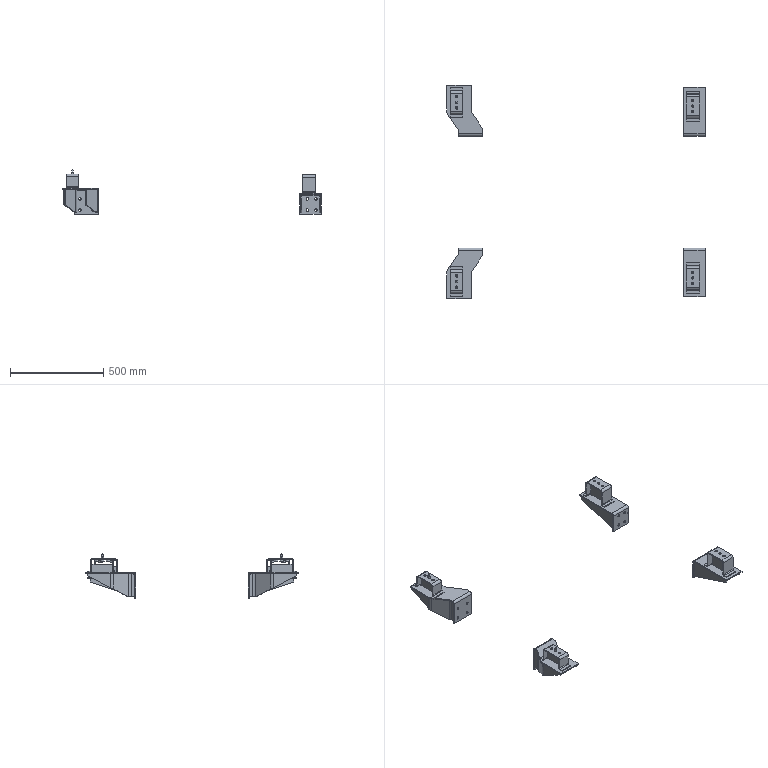Part | NX | features BREP 24 | 30 solids | 676 faces | box 1383 x 1144 x 240 mm | volume 2640420 mm3 | plane 262 | cylinder 176 | cone 118 | spline 64 | torus 56 | commonest cylinder face diameters 12 x48 13 x48 26 x16 20 x12 24 x12 40 x12